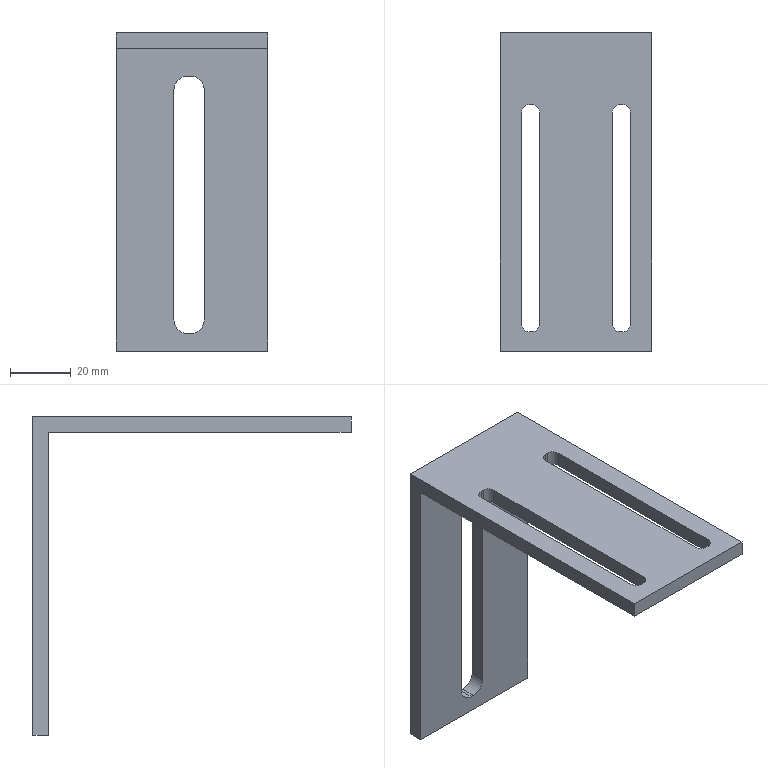Part | SolidWorks | features ICE 3, Extrusion 1 | 1 solid | 32 faces | box 50 x 105 x 105 mm | volume 42641 mm3 | plane 20 | cylinder 12 | commonest cylinder face diameters 5 x8 9 x4
STEP:
#1=CARTESIAN_POINT('',(-25.,50.,0.));
#2=VERTEX_POINT('',#1);
#3=CARTESIAN_POINT('',(-25.,-50.,0.));
#4=VERTEX_POINT('',#3);
#5=CARTESIAN_POINT('',(-25.,-50.,0.));
#6=DIRECTION('',(0.,-1.,0.));
#7=VECTOR('',#6,1000.);
#8=LINE('',#5,#7);
#9=EDGE_CURVE('',#2,#4,#8,.T.);
#10=ORIENTED_EDGE('',*,*,#9,.T.);
#11=CARTESIAN_POINT('',(-25.,-50.,5.));
#12=VERTEX_POINT('',#11);
#13=CARTESIAN_POINT('',(-25.,-50.,5.));
#14=DIRECTION('',(0.,0.,-1.));
#15=VECTOR('',#14,1000.);
#16=LINE('',#13,#15);
#17=EDGE_CURVE('',#12,#4,#16,.T.);
#18=ORIENTED_EDGE('',*,*,#17,.F.);
#19=CARTESIAN_POINT('',(-25.,55.,5.));
#20=VERTEX_POINT('',#19);
#21=CARTESIAN_POINT('',(-25.,-50.,5.));
#22=DIRECTION('',(0.,-1.,0.));
#23=VECTOR('',#22,1000.);
#24=LINE('',#21,#23);
#25=EDGE_CURVE('',#20,#12,#24,.T.);
#26=ORIENTED_EDGE('',*,*,#25,.F.);
#27=CARTESIAN_POINT('',(-25.,55.,-100.));
#28=VERTEX_POINT('',#27);
#29=CARTESIAN_POINT('',(-25.,55.,5.));
#30=DIRECTION('',(0.,0.,-1.));
#31=VECTOR('',#30,1000.);
#32=LINE('',#29,#31);
#33=EDGE_CURVE('',#20,#28,#32,.T.);
#34=ORIENTED_EDGE('',*,*,#33,.T.);
#35=CARTESIAN_POINT('',(-25.,50.,-100.));
#36=VERTEX_POINT('',#35);
#37=CARTESIAN_POINT('',(-25.,50.,-100.));
#38=DIRECTION('',(0.,1.,0.));
#39=VECTOR('',#38,1000.);
#40=LINE('',#37,#39);
#41=EDGE_CURVE('',#36,#28,#40,.T.);
#42=ORIENTED_EDGE('',*,*,#41,.F.);
#43=CARTESIAN_POINT('',(-25.,50.,5.));
#44=DIRECTION('',(0.,0.,-1.));
#45=VECTOR('',#44,1000.);
#46=LINE('',#43,#45);
#47=EDGE_CURVE('',#2,#36,#46,.T.);
#48=ORIENTED_EDGE('',*,*,#47,.F.);
#49=EDGE_LOOP('',(#10,#18,#26,#34,#42,#48));
#50=FACE_OUTER_BOUND('',#49,.T.);
#51=CARTESIAN_POINT('',(-25.,-50.,5.));
#52=DIRECTION('',(1.,0.,0.));
#53=DIRECTION('',(0.,0.,-1.));
#54=AXIS2_PLACEMENT_3D('',#51,#52,#53);
#55=PLANE('',#54);
#56=ADVANCED_FACE('',(#50),#55,.F.);
#57=CARTESIAN_POINT('',(25.,-50.,0.));
#58=VERTEX_POINT('',#57);
#59=CARTESIAN_POINT('',(25.,-50.,0.));
#60=DIRECTION('',(1.,0.,0.));
#61=VECTOR('',#60,1000.);
#62=LINE('',#59,#61);
#63=EDGE_CURVE('',#4,#58,#62,.T.);
#64=ORIENTED_EDGE('',*,*,#63,.T.);
#65=CARTESIAN_POINT('',(25.,-50.,5.));
#66=VERTEX_POINT('',#65);
#67=CARTESIAN_POINT('',(25.,-50.,5.));
#68=DIRECTION('',(0.,0.,-1.));
#69=VECTOR('',#68,1000.);
#70=LINE('',#67,#69);
#71=EDGE_CURVE('',#66,#58,#70,.T.);
#72=ORIENTED_EDGE('',*,*,#71,.F.);
#73=CARTESIAN_POINT('',(25.,-50.,5.));
#74=DIRECTION('',(1.,0.,0.));
#75=VECTOR('',#74,1000.);
#76=LINE('',#73,#75);
#77=EDGE_CURVE('',#12,#66,#76,.T.);
#78=ORIENTED_EDGE('',*,*,#77,.F.);
#79=ORIENTED_EDGE('',*,*,#17,.T.);
#80=EDGE_LOOP('',(#64,#72,#78,#79));
#81=FACE_OUTER_BOUND('',#80,.T.);
#82=CARTESIAN_POINT('',(25.,-50.,5.));
#83=DIRECTION('',(0.,1.,0.));
#84=DIRECTION('',(-1.,0.,0.));
#85=AXIS2_PLACEMENT_3D('',#82,#83,#84);
#86=PLANE('',#85);
#87=ADVANCED_FACE('',(#81),#86,.F.);
#88=CARTESIAN_POINT('',(25.,50.,0.));
#89=VERTEX_POINT('',#88);
#90=CARTESIAN_POINT('',(25.,-50.,0.));
#91=DIRECTION('',(0.,1.,0.));
#92=VECTOR('',#91,1000.);
#93=LINE('',#90,#92);
#94=EDGE_CURVE('',#58,#89,#93,.T.);
#95=ORIENTED_EDGE('',*,*,#94,.T.);
#96=CARTESIAN_POINT('',(25.,50.,-100.));
#97=VERTEX_POINT('',#96);
#98=CARTESIAN_POINT('',(25.,50.,5.));
#99=DIRECTION('',(0.,0.,-1.));
#100=VECTOR('',#99,1000.);
#101=LINE('',#98,#100);
#102=EDGE_CURVE('',#89,#97,#101,.T.);
#103=ORIENTED_EDGE('',*,*,#102,.T.);
#104=CARTESIAN_POINT('',(25.,55.,-100.));
#105=VERTEX_POINT('',#104);
#106=CARTESIAN_POINT('',(25.,50.,-100.));
#107=DIRECTION('',(0.,-1.,0.));
#108=VECTOR('',#107,1000.);
#109=LINE('',#106,#108);
#110=EDGE_CURVE('',#105,#97,#109,.T.);
#111=ORIENTED_EDGE('',*,*,#110,.F.);
#112=CARTESIAN_POINT('',(25.,55.,5.));
#113=VERTEX_POINT('',#112);
#114=CARTESIAN_POINT('',(25.,55.,5.));
#115=DIRECTION('',(0.,0.,-1.));
#116=VECTOR('',#115,1000.);
#117=LINE('',#114,#116);
#118=EDGE_CURVE('',#113,#105,#117,.T.);
#119=ORIENTED_EDGE('',*,*,#118,.F.);
#120=CARTESIAN_POINT('',(25.,-50.,5.));
#121=DIRECTION('',(0.,1.,0.));
#122=VECTOR('',#121,1000.);
#123=LINE('',#120,#122);
#124=EDGE_CURVE('',#66,#113,#123,.T.);
#125=ORIENTED_EDGE('',*,*,#124,.F.);
#126=ORIENTED_EDGE('',*,*,#71,.T.);
#127=EDGE_LOOP('',(#95,#103,#111,#119,#125,#126));
#128=FACE_OUTER_BOUND('',#127,.T.);
#129=CARTESIAN_POINT('',(25.,-50.,5.));
#130=DIRECTION('',(-1.,0.,0.));
#131=DIRECTION('',(0.,0.,1.));
#132=AXIS2_PLACEMENT_3D('',#129,#130,#131);
#133=PLANE('',#132);
#134=ADVANCED_FACE('',(#128),#133,.F.);
#135=CARTESIAN_POINT('',(-18.,-41.155,5.));
#136=VERTEX_POINT('',#135);
#137=CARTESIAN_POINT('',(-15.5,-43.655,5.));
#138=VERTEX_POINT('',#137);
#139=CARTESIAN_POINT('',(-15.5,-41.155,5.));
#140=DIRECTION('',(0.,0.,1.));
#141=DIRECTION('',(-1.,0.,0.));
#142=AXIS2_PLACEMENT_3D('',#139,#140,#141);
#143=CIRCLE('',#142,2.5);
#144=EDGE_CURVE('',#136,#138,#143,.T.);
#145=ORIENTED_EDGE('',*,*,#144,.F.);
#146=CARTESIAN_POINT('',(-18.,28.845,5.));
#147=VERTEX_POINT('',#146);
#148=CARTESIAN_POINT('',(-18.,-41.155,5.));
#149=DIRECTION('',(0.,-1.,0.));
#150=VECTOR('',#149,1000.);
#151=LINE('',#148,#150);
#152=EDGE_CURVE('',#147,#136,#151,.T.);
#153=ORIENTED_EDGE('',*,*,#152,.F.);
#154=CARTESIAN_POINT('',(-15.5,31.345,5.));
#155=VERTEX_POINT('',#154);
#156=CARTESIAN_POINT('',(-15.5,28.845,5.));
#157=DIRECTION('',(0.,0.,1.));
#158=DIRECTION('',(1.,0.,0.));
#159=AXIS2_PLACEMENT_3D('',#156,#157,#158);
#160=CIRCLE('',#159,2.5);
#161=EDGE_CURVE('',#155,#147,#160,.T.);
#162=ORIENTED_EDGE('',*,*,#161,.F.);
#163=CARTESIAN_POINT('',(-14.5,31.345,5.));
#164=VERTEX_POINT('',#163);
#165=CARTESIAN_POINT('',(-14.5,31.345,5.));
#166=DIRECTION('',(-1.,0.,0.));
#167=VECTOR('',#166,1000.);
#168=LINE('',#165,#167);
#169=EDGE_CURVE('',#164,#155,#168,.T.);
#170=ORIENTED_EDGE('',*,*,#169,.F.);
#171=CARTESIAN_POINT('',(-12.,28.845,5.));
#172=VERTEX_POINT('',#171);
#173=CARTESIAN_POINT('',(-14.5,28.845,5.));
#174=DIRECTION('',(0.,0.,1.));
#175=DIRECTION('',(1.,0.,0.));
#176=AXIS2_PLACEMENT_3D('',#173,#174,#175);
#177=CIRCLE('',#176,2.5);
#178=EDGE_CURVE('',#172,#164,#177,.T.);
#179=ORIENTED_EDGE('',*,*,#178,.F.);
#180=CARTESIAN_POINT('',(-12.,-41.155,5.));
#181=VERTEX_POINT('',#180);
#182=CARTESIAN_POINT('',(-12.,-41.155,5.));
#183=DIRECTION('',(0.,1.,0.));
#184=VECTOR('',#183,1000.);
#185=LINE('',#182,#184);
#186=EDGE_CURVE('',#181,#172,#185,.T.);
#187=ORIENTED_EDGE('',*,*,#186,.F.);
#188=CARTESIAN_POINT('',(-14.5,-43.655,5.));
#189=VERTEX_POINT('',#188);
#190=CARTESIAN_POINT('',(-14.5,-41.155,5.));
#191=DIRECTION('',(0.,0.,1.));
#192=DIRECTION('',(1.,0.,0.));
#193=AXIS2_PLACEMENT_3D('',#190,#191,#192);
#194=CIRCLE('',#193,2.5);
#195=EDGE_CURVE('',#189,#181,#194,.T.);
#196=ORIENTED_EDGE('',*,*,#195,.F.);
#197=CARTESIAN_POINT('',(-14.5,-43.655,5.));
#198=DIRECTION('',(1.,0.,0.));
#199=VECTOR('',#198,1000.);
#200=LINE('',#197,#199);
#201=EDGE_CURVE('',#138,#189,#200,.T.);
#202=ORIENTED_EDGE('',*,*,#201,.F.);
#203=EDGE_LOOP('',(#145,#153,#162,#170,#179,#187,#196,#202));
#204=FACE_BOUND('',#203,.T.);
#205=CARTESIAN_POINT('',(14.5,31.345,5.));
#206=VERTEX_POINT('',#205);
#207=CARTESIAN_POINT('',(12.,28.845,5.));
#208=VERTEX_POINT('',#207);
#209=CARTESIAN_POINT('',(14.5,28.845,5.));
#210=DIRECTION('',(0.,0.,1.));
#211=DIRECTION('',(1.,0.,0.));
#212=AXIS2_PLACEMENT_3D('',#209,#210,#211);
#213=CIRCLE('',#212,2.5);
#214=EDGE_CURVE('',#206,#208,#213,.T.);
#215=ORIENTED_EDGE('',*,*,#214,.F.);
#216=CARTESIAN_POINT('',(15.5,31.345,5.));
#217=VERTEX_POINT('',#216);
#218=CARTESIAN_POINT('',(15.5,31.345,5.));
#219=DIRECTION('',(-1.,0.,0.));
#220=VECTOR('',#219,1000.);
#221=LINE('',#218,#220);
#222=EDGE_CURVE('',#217,#206,#221,.T.);
#223=ORIENTED_EDGE('',*,*,#222,.F.);
#224=CARTESIAN_POINT('',(18.,28.845,5.));
#225=VERTEX_POINT('',#224);
#226=CARTESIAN_POINT('',(15.5,28.845,5.));
#227=DIRECTION('',(0.,0.,1.));
#228=DIRECTION('',(1.,0.,0.));
#229=AXIS2_PLACEMENT_3D('',#226,#227,#228);
#230=CIRCLE('',#229,2.5);
#231=EDGE_CURVE('',#225,#217,#230,.T.);
#232=ORIENTED_EDGE('',*,*,#231,.F.);
#233=CARTESIAN_POINT('',(18.,-41.155,5.));
#234=VERTEX_POINT('',#233);
#235=CARTESIAN_POINT('',(18.,-41.155,5.));
#236=DIRECTION('',(0.,1.,0.));
#237=VECTOR('',#236,1000.);
#238=LINE('',#235,#237);
#239=EDGE_CURVE('',#234,#225,#238,.T.);
#240=ORIENTED_EDGE('',*,*,#239,.F.);
#241=CARTESIAN_POINT('',(15.5,-43.655,5.));
#242=VERTEX_POINT('',#241);
#243=CARTESIAN_POINT('',(15.5,-41.155,5.));
#244=DIRECTION('',(0.,0.,1.));
#245=DIRECTION('',(1.,0.,0.));
#246=AXIS2_PLACEMENT_3D('',#243,#244,#245);
#247=CIRCLE('',#246,2.5);
#248=EDGE_CURVE('',#242,#234,#247,.T.);
#249=ORIENTED_EDGE('',*,*,#248,.F.);
#250=CARTESIAN_POINT('',(14.5,-43.655,5.));
#251=VERTEX_POINT('',#250);
#252=CARTESIAN_POINT('',(15.5,-43.655,5.));
#253=DIRECTION('',(1.,0.,0.));
#254=VECTOR('',#253,1000.);
#255=LINE('',#252,#254);
#256=EDGE_CURVE('',#251,#242,#255,.T.);
#257=ORIENTED_EDGE('',*,*,#256,.F.);
#258=CARTESIAN_POINT('',(12.,-41.155,5.));
#259=VERTEX_POINT('',#258);
#260=CARTESIAN_POINT('',(14.5,-41.155,5.));
#261=DIRECTION('',(0.,0.,1.));
#262=DIRECTION('',(-1.,0.,0.));
#263=AXIS2_PLACEMENT_3D('',#260,#261,#262);
#264=CIRCLE('',#263,2.5);
#265=EDGE_CURVE('',#259,#251,#264,.T.);
#266=ORIENTED_EDGE('',*,*,#265,.F.);
#267=CARTESIAN_POINT('',(12.,-41.155,5.));
#268=DIRECTION('',(0.,-1.,0.));
#269=VECTOR('',#268,1000.);
#270=LINE('',#267,#269);
#271=EDGE_CURVE('',#208,#259,#270,.T.);
#272=ORIENTED_EDGE('',*,*,#271,.F.);
#273=EDGE_LOOP('',(#215,#223,#232,#240,#249,#257,#266,#272));
#274=FACE_BOUND('',#273,.T.);
#275=ORIENTED_EDGE('',*,*,#25,.T.);
#276=ORIENTED_EDGE('',*,*,#77,.T.);
#277=ORIENTED_EDGE('',*,*,#124,.T.);
#278=CARTESIAN_POINT('',(-25.,55.,5.));
#279=DIRECTION('',(1.,0.,0.));
#280=VECTOR('',#279,1000.);
#281=LINE('',#278,#280);
#282=EDGE_CURVE('',#20,#113,#281,.T.);
#283=ORIENTED_EDGE('',*,*,#282,.F.);
#284=EDGE_LOOP('',(#275,#276,#277,#283));
#285=FACE_OUTER_BOUND('',#284,.T.);
#286=CARTESIAN_POINT('',(-25.,50.,5.));
#287=DIRECTION('',(0.,0.,1.));
#288=DIRECTION('',(1.,0.,0.));
#289=AXIS2_PLACEMENT_3D('',#286,#287,#288);
#290=PLANE('',#289);
#291=ADVANCED_FACE('',(#204,#274,#285),#290,.T.);
#292=CARTESIAN_POINT('',(-18.,28.845,0.));
#293=VERTEX_POINT('',#292);
#294=CARTESIAN_POINT('',(-18.,-41.155,0.));
#295=VERTEX_POINT('',#294);
#296=CARTESIAN_POINT('',(-18.,50.,0.));
#297=DIRECTION('',(0.,-1.,0.));
#298=VECTOR('',#297,1000.);
#299=LINE('',#296,#298);
#300=EDGE_CURVE('',#293,#295,#299,.T.);
#301=ORIENTED_EDGE('',*,*,#300,.T.);
#302=CARTESIAN_POINT('',(-15.5,-43.655,0.));
#303=VERTEX_POINT('',#302);
#304=CARTESIAN_POINT('',(-15.5,-41.155,0.));
#305=DIRECTION('',(0.,0.,1.));
#306=DIRECTION('',(1.,0.,0.));
#307=AXIS2_PLACEMENT_3D('',#304,#305,#306);
#308=CIRCLE('',#307,2.5);
#309=EDGE_CURVE('',#295,#303,#308,.T.);
#310=ORIENTED_EDGE('',*,*,#309,.T.);
#311=CARTESIAN_POINT('',(-14.5,-43.655,0.));
#312=VERTEX_POINT('',#311);
#313=CARTESIAN_POINT('',(-25.,-43.655,0.));
#314=DIRECTION('',(1.,0.,0.));
#315=VECTOR('',#314,1000.);
#316=LINE('',#313,#315);
#317=EDGE_CURVE('',#303,#312,#316,.T.);
#318=ORIENTED_EDGE('',*,*,#317,.T.);
#319=CARTESIAN_POINT('',(-12.,-41.155,0.));
#320=VERTEX_POINT('',#319);
#321=CARTESIAN_POINT('',(-14.5,-41.155,0.));
#322=DIRECTION('',(0.,0.,1.));
#323=DIRECTION('',(1.,0.,0.));
#324=AXIS2_PLACEMENT_3D('',#321,#322,#323);
#325=CIRCLE('',#324,2.5);
#326=EDGE_CURVE('',#312,#320,#325,.T.);
#327=ORIENTED_EDGE('',*,*,#326,.T.);
#328=CARTESIAN_POINT('',(-12.,28.845,0.));
#329=VERTEX_POINT('',#328);
#330=CARTESIAN_POINT('',(-12.,50.,0.));
#331=DIRECTION('',(0.,1.,0.));
#332=VECTOR('',#331,1000.);
#333=LINE('',#330,#332);
#334=EDGE_CURVE('',#320,#329,#333,.T.);
#335=ORIENTED_EDGE('',*,*,#334,.T.);
#336=CARTESIAN_POINT('',(-14.5,31.345,0.));
#337=VERTEX_POINT('',#336);
#338=CARTESIAN_POINT('',(-14.5,28.845,0.));
#339=DIRECTION('',(0.,0.,1.));
#340=DIRECTION('',(1.,0.,0.));
#341=AXIS2_PLACEMENT_3D('',#338,#339,#340);
#342=CIRCLE('',#341,2.5);
#343=EDGE_CURVE('',#329,#337,#342,.T.);
#344=ORIENTED_EDGE('',*,*,#343,.T.);
#345=CARTESIAN_POINT('',(-15.5,31.345,0.));
#346=VERTEX_POINT('',#345);
#347=CARTESIAN_POINT('',(-25.,31.345,0.));
#348=DIRECTION('',(-1.,0.,0.));
#349=VECTOR('',#348,1000.);
#350=LINE('',#347,#349);
#351=EDGE_CURVE('',#337,#346,#350,.T.);
#352=ORIENTED_EDGE('',*,*,#351,.T.);
#353=CARTESIAN_POINT('',(-15.5,28.845,0.));
#354=DIRECTION('',(0.,0.,1.));
#355=DIRECTION('',(1.,0.,0.));
#356=AXIS2_PLACEMENT_3D('',#353,#354,#355);
#357=CIRCLE('',#356,2.5);
#358=EDGE_CURVE('',#346,#293,#357,.T.);
#359=ORIENTED_EDGE('',*,*,#358,.T.);
#360=EDGE_LOOP('',(#301,#310,#318,#327,#335,#344,#352,#359));
#361=FACE_BOUND('',#360,.T.);
#362=CARTESIAN_POINT('',(15.5,31.345,0.));
#363=VERTEX_POINT('',#362);
#364=CARTESIAN_POINT('',(14.5,31.345,0.));
#365=VERTEX_POINT('',#364);
#366=CARTESIAN_POINT('',(-25.,31.345,0.));
#367=DIRECTION('',(-1.,0.,0.));
#368=VECTOR('',#367,1000.);
#369=LINE('',#366,#368);
#370=EDGE_CURVE('',#363,#365,#369,.T.);
#371=ORIENTED_EDGE('',*,*,#370,.T.);
#372=CARTESIAN_POINT('',(12.,28.845,0.));
#373=VERTEX_POINT('',#372);
#374=CARTESIAN_POINT('',(14.5,28.845,0.));
#375=DIRECTION('',(0.,0.,1.));
#376=DIRECTION('',(1.,0.,0.));
#377=AXIS2_PLACEMENT_3D('',#374,#375,#376);
#378=CIRCLE('',#377,2.5);
#379=EDGE_CURVE('',#365,#373,#378,.T.);
#380=ORIENTED_EDGE('',*,*,#379,.T.);
#381=CARTESIAN_POINT('',(12.,-41.155,0.));
#382=VERTEX_POINT('',#381);
#383=CARTESIAN_POINT('',(12.,50.,0.));
#384=DIRECTION('',(0.,-1.,0.));
#385=VECTOR('',#384,1000.);
#386=LINE('',#383,#385);
#387=EDGE_CURVE('',#373,#382,#386,.T.);
#388=ORIENTED_EDGE('',*,*,#387,.T.);
#389=CARTESIAN_POINT('',(14.5,-43.655,0.));
#390=VERTEX_POINT('',#389);
#391=CARTESIAN_POINT('',(14.5,-41.155,0.));
#392=DIRECTION('',(0.,0.,1.));
#393=DIRECTION('',(1.,0.,0.));
#394=AXIS2_PLACEMENT_3D('',#391,#392,#393);
#395=CIRCLE('',#394,2.5);
#396=EDGE_CURVE('',#382,#390,#395,.T.);
#397=ORIENTED_EDGE('',*,*,#396,.T.);
#398=CARTESIAN_POINT('',(15.5,-43.655,0.));
#399=VERTEX_POINT('',#398);
#400=CARTESIAN_POINT('',(-25.,-43.655,0.));
#401=DIRECTION('',(1.,0.,0.));
#402=VECTOR('',#401,1000.);
#403=LINE('',#400,#402);
#404=EDGE_CURVE('',#390,#399,#403,.T.);
#405=ORIENTED_EDGE('',*,*,#404,.T.);
#406=CARTESIAN_POINT('',(18.,-41.155,0.));
#407=VERTEX_POINT('',#406);
#408=CARTESIAN_POINT('',(15.5,-41.155,0.));
#409=DIRECTION('',(0.,0.,1.));
#410=DIRECTION('',(1.,0.,0.));
#411=AXIS2_PLACEMENT_3D('',#408,#409,#410);
#412=CIRCLE('',#411,2.5);
#413=EDGE_CURVE('',#399,#407,#412,.T.);
#414=ORIENTED_EDGE('',*,*,#413,.T.);
#415=CARTESIAN_POINT('',(18.,28.845,0.));
#416=VERTEX_POINT('',#415);
#417=CARTESIAN_POINT('',(18.,50.,0.));
#418=DIRECTION('',(0.,1.,0.));
#419=VECTOR('',#418,1000.);
#420=LINE('',#417,#419);
#421=EDGE_CURVE('',#407,#416,#420,.T.);
#422=ORIENTED_EDGE('',*,*,#421,.T.);
#423=CARTESIAN_POINT('',(15.5,28.845,0.));
#424=DIRECTION('',(0.,0.,1.));
#425=DIRECTION('',(1.,0.,0.));
#426=AXIS2_PLACEMENT_3D('',#423,#424,#425);
#427=CIRCLE('',#426,2.5);
#428=EDGE_CURVE('',#416,#363,#427,.T.);
#429=ORIENTED_EDGE('',*,*,#428,.T.);
#430=EDGE_LOOP('',(#371,#380,#388,#397,#405,#414,#422,#429));
#431=FACE_BOUND('',#430,.T.);
#432=ORIENTED_EDGE('',*,*,#9,.F.);
#433=CARTESIAN_POINT('',(25.,50.,0.));
#434=DIRECTION('',(-1.,0.,0.));
#435=VECTOR('',#434,1000.);
#436=LINE('',#433,#435);
#437=EDGE_CURVE('',#89,#2,#436,.T.);
#438=ORIENTED_EDGE('',*,*,#437,.F.);
#439=ORIENTED_EDGE('',*,*,#94,.F.);
#440=ORIENTED_EDGE('',*,*,#63,.F.);
#441=EDGE_LOOP('',(#432,#438,#439,#440));
#442=FACE_OUTER_BOUND('',#441,.T.);
#443=CARTESIAN_POINT('',(-25.,50.,0.));
#444=DIRECTION('',(0.,0.,1.));
#445=DIRECTION('',(1.,0.,0.));
#446=AXIS2_PLACEMENT_3D('',#443,#444,#445);
#447=PLANE('',#446);
#448=ADVANCED_FACE('',(#361,#431,#442),#447,.F.);
#449=CARTESIAN_POINT('',(14.5,31.345,-5.));
#450=DIRECTION('',(0.,0.,1.));
#451=VECTOR('',#450,1000.);
#452=LINE('',#449,#451);
#453=EDGE_CURVE('',#365,#206,#452,.T.);
#454=ORIENTED_EDGE('',*,*,#453,.T.);
#455=ORIENTED_EDGE('',*,*,#214,.T.);
#456=CARTESIAN_POINT('',(12.,28.845,-5.));
#457=DIRECTION('',(0.,0.,1.));
#458=VECTOR('',#457,1000.);
#459=LINE('',#456,#458);
#460=EDGE_CURVE('',#373,#208,#459,.T.);
#461=ORIENTED_EDGE('',*,*,#460,.F.);
#462=ORIENTED_EDGE('',*,*,#379,.F.);
#463=EDGE_LOOP('',(#454,#455,#461,#462));
#464=FACE_OUTER_BOUND('',#463,.T.);
#465=CARTESIAN_POINT('',(14.5,28.845,-5.));
#466=DIRECTION('',(0.,0.,1.));
#467=DIRECTION('',(1.,0.,0.));
#468=AXIS2_PLACEMENT_3D('',#465,#466,#467);
#469=CYLINDRICAL_SURFACE('',#468,2.5);
#470=ADVANCED_FACE('',(#464),#469,.F.);
#471=CARTESIAN_POINT('',(15.5,31.345,-5.));
#472=DIRECTION('',(0.,0.,1.));
#473=VECTOR('',#472,1000.);
#474=LINE('',#471,#473);
#475=EDGE_CURVE('',#363,#217,#474,.T.);
#476=ORIENTED_EDGE('',*,*,#475,.T.);
#477=ORIENTED_EDGE('',*,*,#222,.T.);
#478=ORIENTED_EDGE('',*,*,#453,.F.);
#479=ORIENTED_EDGE('',*,*,#370,.F.);
#480=EDGE_LOOP('',(#476,#477,#478,#479));
#481=FACE_OUTER_BOUND('',#480,.T.);
#482=CARTESIAN_POINT('',(15.5,31.345,-5.));
#483=DIRECTION('',(0.,1.,0.));
#484=DIRECTION('',(0.,0.,1.));
#485=AXIS2_PLACEMENT_3D('',#482,#483,#484);
#486=PLANE('',#485);
#487=ADVANCED_FACE('',(#481),#486,.F.);
#488=CARTESIAN_POINT('',(18.,28.845,-5.));
#489=DIRECTION('',(0.,0.,1.));
#490=VECTOR('',#489,1000.);
#491=LINE('',#488,#490);
#492=EDGE_CURVE('',#416,#225,#491,.T.);
#493=ORIENTED_EDGE('',*,*,#492,.T.);
#494=ORIENTED_EDGE('',*,*,#231,.T.);
#495=ORIENTED_EDGE('',*,*,#475,.F.);
#496=ORIENTED_EDGE('',*,*,#428,.F.);
#497=EDGE_LOOP('',(#493,#494,#495,#496));
#498=FACE_OUTER_BOUND('',#497,.T.);
#499=CARTESIAN_POINT('',(15.5,28.845,-5.));
#500=DIRECTION('',(0.,0.,1.));
#501=DIRECTION('',(1.,0.,0.));
#502=AXIS2_PLACEMENT_3D('',#499,#500,#501);
#503=CYLINDRICAL_SURFACE('',#502,2.5);
#504=ADVANCED_FACE('',(#498),#503,.F.);
#505=CARTESIAN_POINT('',(18.,-41.155,-5.));
#506=DIRECTION('',(0.,0.,1.));
#507=VECTOR('',#506,1000.);
#508=LINE('',#505,#507);
#509=EDGE_CURVE('',#407,#234,#508,.T.);
#510=ORIENTED_EDGE('',*,*,#509,.T.);
#511=ORIENTED_EDGE('',*,*,#239,.T.);
#512=ORIENTED_EDGE('',*,*,#492,.F.);
#513=ORIENTED_EDGE('',*,*,#421,.F.);
#514=EDGE_LOOP('',(#510,#511,#512,#513));
#515=FACE_OUTER_BOUND('',#514,.T.);
#516=CARTESIAN_POINT('',(18.,-41.155,-5.));
#517=DIRECTION('',(1.,0.,0.));
#518=DIRECTION('',(0.,0.,-1.));
#519=AXIS2_PLACEMENT_3D('',#516,#517,#518);
#520=PLANE('',#519);
#521=ADVANCED_FACE('',(#515),#520,.F.);
#522=CARTESIAN_POINT('',(15.5,-43.655,-5.));
#523=DIRECTION('',(0.,0.,1.));
#524=VECTOR('',#523,1000.);
#525=LINE('',#522,#524);
#526=EDGE_CURVE('',#399,#242,#525,.T.);
#527=ORIENTED_EDGE('',*,*,#526,.T.);
#528=ORIENTED_EDGE('',*,*,#248,.T.);
#529=ORIENTED_EDGE('',*,*,#509,.F.);
#530=ORIENTED_EDGE('',*,*,#413,.F.);
#531=EDGE_LOOP('',(#527,#528,#529,#530));
#532=FACE_OUTER_BOUND('',#531,.T.);
#533=CARTESIAN_POINT('',(15.5,-41.155,-5.));
#534=DIRECTION('',(0.,0.,1.));
#535=DIRECTION('',(1.,0.,0.));
#536=AXIS2_PLACEMENT_3D('',#533,#534,#535);
#537=CYLINDRICAL_SURFACE('',#536,2.5);
#538=ADVANCED_FACE('',(#532),#537,.F.);
#539=CARTESIAN_POINT('',(14.5,-43.655,-5.));
#540=DIRECTION('',(0.,0.,1.));
#541=VECTOR('',#540,1000.);
#542=LINE('',#539,#541);
#543=EDGE_CURVE('',#390,#251,#542,.T.);
#544=ORIENTED_EDGE('',*,*,#543,.T.);
#545=ORIENTED_EDGE('',*,*,#256,.T.);
#546=ORIENTED_EDGE('',*,*,#526,.F.);
#547=ORIENTED_EDGE('',*,*,#404,.F.);
#548=EDGE_LOOP('',(#544,#545,#546,#547));
#549=FACE_OUTER_BOUND('',#548,.T.);
#550=CARTESIAN_POINT('',(15.5,-43.655,-5.));
#551=DIRECTION('',(0.,-1.,0.));
#552=DIRECTION('',(0.,0.,-1.));
#553=AXIS2_PLACEMENT_3D('',#550,#551,#552);
#554=PLANE('',#553);
#555=ADVANCED_FACE('',(#549),#554,.F.);
#556=CARTESIAN_POINT('',(12.,-41.155,-5.));
#557=DIRECTION('',(0.,0.,1.));
#558=VECTOR('',#557,1000.);
#559=LINE('',#556,#558);
#560=EDGE_CURVE('',#382,#259,#559,.T.);
#561=ORIENTED_EDGE('',*,*,#560,.T.);
#562=ORIENTED_EDGE('',*,*,#265,.T.);
#563=ORIENTED_EDGE('',*,*,#543,.F.);
#564=ORIENTED_EDGE('',*,*,#396,.F.);
#565=EDGE_LOOP('',(#561,#562,#563,#564));
#566=FACE_OUTER_BOUND('',#565,.T.);
#567=CARTESIAN_POINT('',(14.5,-41.155,-5.));
#568=DIRECTION('',(0.,0.,1.));
#569=DIRECTION('',(1.,0.,0.));
#570=AXIS2_PLACEMENT_3D('',#567,#568,#569);
#571=CYLINDRICAL_SURFACE('',#570,2.5);
#572=ADVANCED_FACE('',(#566),#571,.F.);
#573=ORIENTED_EDGE('',*,*,#460,.T.);
#574=ORIENTED_EDGE('',*,*,#271,.T.);
#575=ORIENTED_EDGE('',*,*,#560,.F.);
#576=ORIENTED_EDGE('',*,*,#387,.F.);
#577=EDGE_LOOP('',(#573,#574,#575,#576));
#578=FACE_OUTER_BOUND('',#577,.T.);
#579=CARTESIAN_POINT('',(12.,-41.155,-5.));
#580=DIRECTION('',(-1.,0.,0.));
#581=DIRECTION('',(0.,0.,1.));
#582=AXIS2_PLACEMENT_3D('',#579,#580,#581);
#583=PLANE('',#582);
#584=ADVANCED_FACE('',(#578),#583,.F.);
#585=CARTESIAN_POINT('',(-18.,-41.155,-5.));
#586=DIRECTION('',(0.,0.,1.));
#587=VECTOR('',#586,1000.);
#588=LINE('',#585,#587);
#589=EDGE_CURVE('',#295,#136,#588,.T.);
#590=ORIENTED_EDGE('',*,*,#589,.T.);
#591=ORIENTED_EDGE('',*,*,#144,.T.);
#592=CARTESIAN_POINT('',(-15.5,-43.655,-5.));
#593=DIRECTION('',(0.,0.,1.));
#594=VECTOR('',#593,1000.);
#595=LINE('',#592,#594);
#596=EDGE_CURVE('',#303,#138,#595,.T.);
#597=ORIENTED_EDGE('',*,*,#596,.F.);
#598=ORIENTED_EDGE('',*,*,#309,.F.);
#599=EDGE_LOOP('',(#590,#591,#597,#598));
#600=FACE_OUTER_BOUND('',#599,.T.);
#601=CARTESIAN_POINT('',(-15.5,-41.155,-5.));
#602=DIRECTION('',(0.,0.,1.));
#603=DIRECTION('',(1.,0.,0.));
#604=AXIS2_PLACEMENT_3D('',#601,#602,#603);
#605=CYLINDRICAL_SURFACE('',#604,2.5);
#606=ADVANCED_FACE('',(#600),#605,.F.);
#607=CARTESIAN_POINT('',(-18.,28.845,-5.));
#608=DIRECTION('',(0.,0.,1.));
#609=VECTOR('',#608,1000.);
#610=LINE('',#607,#609);
#611=EDGE_CURVE('',#293,#147,#610,.T.);
#612=ORIENTED_EDGE('',*,*,#611,.T.);
#613=ORIENTED_EDGE('',*,*,#152,.T.);
#614=ORIENTED_EDGE('',*,*,#589,.F.);
#615=ORIENTED_EDGE('',*,*,#300,.F.);
#616=EDGE_LOOP('',(#612,#613,#614,#615));
#617=FACE_OUTER_BOUND('',#616,.T.);
#618=CARTESIAN_POINT('',(-18.,-41.155,-5.));
#619=DIRECTION('',(-1.,0.,0.));
#620=DIRECTION('',(0.,0.,1.));
#621=AXIS2_PLACEMENT_3D('',#618,#619,#620);
#622=PLANE('',#621);
#623=ADVANCED_FACE('',(#617),#622,.F.);
#624=CARTESIAN_POINT('',(-15.5,31.345,-5.));
#625=DIRECTION('',(0.,0.,1.));
#626=VECTOR('',#625,1000.);
#627=LINE('',#624,#626);
#628=EDGE_CURVE('',#346,#155,#627,.T.);
#629=ORIENTED_EDGE('',*,*,#628,.T.);
#630=ORIENTED_EDGE('',*,*,#161,.T.);
#631=ORIENTED_EDGE('',*,*,#611,.F.);
#632=ORIENTED_EDGE('',*,*,#358,.F.);
#633=EDGE_LOOP('',(#629,#630,#631,#632));
#634=FACE_OUTER_BOUND('',#633,.T.);
#635=CARTESIAN_POINT('',(-15.5,28.845,-5.));
#636=DIRECTION('',(0.,0.,1.));
#637=DIRECTION('',(1.,0.,0.));
#638=AXIS2_PLACEMENT_3D('',#635,#636,#637);
#639=CYLINDRICAL_SURFACE('',#638,2.5);
#640=ADVANCED_FACE('',(#634),#639,.F.);
#641=CARTESIAN_POINT('',(-14.5,31.345,-5.));
#642=DIRECTION('',(0.,0.,1.));
#643=VECTOR('',#642,1000.);
#644=LINE('',#641,#643);
#645=EDGE_CURVE('',#337,#164,#644,.T.);
#646=ORIENTED_EDGE('',*,*,#645,.T.);
#647=ORIENTED_EDGE('',*,*,#169,.T.);
#648=ORIENTED_EDGE('',*,*,#628,.F.);
#649=ORIENTED_EDGE('',*,*,#351,.F.);
#650=EDGE_LOOP('',(#646,#647,#648,#649));
#651=FACE_OUTER_BOUND('',#650,.T.);
#652=CARTESIAN_POINT('',(-14.5,31.345,-5.));
#653=DIRECTION('',(0.,1.,0.));
#654=DIRECTION('',(0.,0.,1.));
#655=AXIS2_PLACEMENT_3D('',#652,#653,#654);
#656=PLANE('',#655);
#657=ADVANCED_FACE('',(#651),#656,.F.);
#658=CARTESIAN_POINT('',(-12.,28.845,-5.));
#659=DIRECTION('',(0.,0.,1.));
#660=VECTOR('',#659,1000.);
#661=LINE('',#658,#660);
#662=EDGE_CURVE('',#329,#172,#661,.T.);
#663=ORIENTED_EDGE('',*,*,#662,.T.);
#664=ORIENTED_EDGE('',*,*,#178,.T.);
#665=ORIENTED_EDGE('',*,*,#645,.F.);
#666=ORIENTED_EDGE('',*,*,#343,.F.);
#667=EDGE_LOOP('',(#663,#664,#665,#666));
#668=FACE_OUTER_BOUND('',#667,.T.);
#669=CARTESIAN_POINT('',(-14.5,28.845,-5.));
#670=DIRECTION('',(0.,0.,1.));
#671=DIRECTION('',(1.,0.,0.));
#672=AXIS2_PLACEMENT_3D('',#669,#670,#671);
#673=CYLINDRICAL_SURFACE('',#672,2.5);
#674=ADVANCED_FACE('',(#668),#673,.F.);
#675=CARTESIAN_POINT('',(-12.,-41.155,-5.));
#676=DIRECTION('',(0.,0.,1.));
#677=VECTOR('',#676,1000.);
#678=LINE('',#675,#677);
#679=EDGE_CURVE('',#320,#181,#678,.T.);
#680=ORIENTED_EDGE('',*,*,#679,.T.);
#681=ORIENTED_EDGE('',*,*,#186,.T.);
#682=ORIENTED_EDGE('',*,*,#662,.F.);
#683=ORIENTED_EDGE('',*,*,#334,.F.);
#684=EDGE_LOOP('',(#680,#681,#682,#683));
#685=FACE_OUTER_BOUND('',#684,.T.);
#686=CARTESIAN_POINT('',(-12.,-41.155,-5.));
#687=DIRECTION('',(1.,0.,0.));
#688=DIRECTION('',(0.,0.,-1.));
#689=AXIS2_PLACEMENT_3D('',#686,#687,#688);
#690=PLANE('',#689);
#691=ADVANCED_FACE('',(#685),#690,.F.);
#692=CARTESIAN_POINT('',(-14.5,-43.655,-5.));
#693=DIRECTION('',(0.,0.,1.));
#694=VECTOR('',#693,1000.);
#695=LINE('',#692,#694);
#696=EDGE_CURVE('',#312,#189,#695,.T.);
#697=ORIENTED_EDGE('',*,*,#696,.T.);
#698=ORIENTED_EDGE('',*,*,#195,.T.);
#699=ORIENTED_EDGE('',*,*,#679,.F.);
#700=ORIENTED_EDGE('',*,*,#326,.F.);
#701=EDGE_LOOP('',(#697,#698,#699,#700));
#702=FACE_OUTER_BOUND('',#701,.T.);
#703=CARTESIAN_POINT('',(-14.5,-41.155,-5.));
#704=DIRECTION('',(0.,0.,1.));
#705=DIRECTION('',(1.,0.,0.));
#706=AXIS2_PLACEMENT_3D('',#703,#704,#705);
#707=CYLINDRICAL_SURFACE('',#706,2.5);
#708=ADVANCED_FACE('',(#702),#707,.F.);
#709=ORIENTED_EDGE('',*,*,#596,.T.);
#710=ORIENTED_EDGE('',*,*,#201,.T.);
#711=ORIENTED_EDGE('',*,*,#696,.F.);
#712=ORIENTED_EDGE('',*,*,#317,.F.);
#713=EDGE_LOOP('',(#709,#710,#711,#712));
#714=FACE_OUTER_BOUND('',#713,.T.);
#715=CARTESIAN_POINT('',(-14.5,-43.655,-5.));
#716=DIRECTION('',(0.,-1.,0.));
#717=DIRECTION('',(0.,0.,-1.));
#718=AXIS2_PLACEMENT_3D('',#715,#716,#717);
#719=PLANE('',#718);
#720=ADVANCED_FACE('',(#714),#719,.F.);
#721=CARTESIAN_POINT('',(-5.974,50.,-89.753));
#722=VERTEX_POINT('',#721);
#723=CARTESIAN_POINT('',(-1.474,50.,-94.253));
#724=VERTEX_POINT('',#723);
#725=CARTESIAN_POINT('',(-1.474,50.,-89.753));
#726=DIRECTION('',(0.,-1.,0.));
#727=DIRECTION('',(-1.,0.,0.));
#728=AXIS2_PLACEMENT_3D('',#725,#726,#727);
#729=CIRCLE('',#728,4.5);
#730=EDGE_CURVE('',#722,#724,#729,.T.);
#731=ORIENTED_EDGE('',*,*,#730,.F.);
#732=CARTESIAN_POINT('',(-5.974,50.,-13.753));
#733=VERTEX_POINT('',#732);
#734=CARTESIAN_POINT('',(-5.974,50.,-89.753));
#735=DIRECTION('',(0.,0.,-1.));
#736=VECTOR('',#735,1000.);
#737=LINE('',#734,#736);
#738=EDGE_CURVE('',#733,#722,#737,.T.);
#739=ORIENTED_EDGE('',*,*,#738,.F.);
#740=CARTESIAN_POINT('',(-1.474,50.,-9.253));
#741=VERTEX_POINT('',#740);
#742=CARTESIAN_POINT('',(-1.474,50.,-13.753));
#743=DIRECTION('',(0.,-1.,0.));
#744=DIRECTION('',(1.,0.,0.));
#745=AXIS2_PLACEMENT_3D('',#742,#743,#744);
#746=CIRCLE('',#745,4.5);
#747=EDGE_CURVE('',#741,#733,#746,.T.);
#748=ORIENTED_EDGE('',*,*,#747,.F.);
#749=CARTESIAN_POINT('',(-0.474,50.,-9.253));
#750=VERTEX_POINT('',#749);
#751=CARTESIAN_POINT('',(-0.474,50.,-9.253));
#752=DIRECTION('',(-1.,0.,0.));
#753=VECTOR('',#752,1000.);
#754=LINE('',#751,#753);
#755=EDGE_CURVE('',#750,#741,#754,.T.);
#756=ORIENTED_EDGE('',*,*,#755,.F.);
#757=CARTESIAN_POINT('',(4.026,50.,-13.753));
#758=VERTEX_POINT('',#757);
#759=CARTESIAN_POINT('',(-0.474,50.,-13.753));
#760=DIRECTION('',(0.,-1.,0.));
#761=DIRECTION('',(1.,0.,0.));
#762=AXIS2_PLACEMENT_3D('',#759,#760,#761);
#763=CIRCLE('',#762,4.5);
#764=EDGE_CURVE('',#758,#750,#763,.T.);
#765=ORIENTED_EDGE('',*,*,#764,.F.);
#766=CARTESIAN_POINT('',(4.026,50.,-89.753));
#767=VERTEX_POINT('',#766);
#768=CARTESIAN_POINT('',(4.026,50.,-89.753));
#769=DIRECTION('',(0.,0.,1.));
#770=VECTOR('',#769,1000.);
#771=LINE('',#768,#770);
#772=EDGE_CURVE('',#767,#758,#771,.T.);
#773=ORIENTED_EDGE('',*,*,#772,.F.);
#774=CARTESIAN_POINT('',(-0.474,50.,-94.253));
#775=VERTEX_POINT('',#774);
#776=CARTESIAN_POINT('',(-0.474,50.,-89.753));
#777=DIRECTION('',(0.,-1.,0.));
#778=DIRECTION('',(1.,0.,0.));
#779=AXIS2_PLACEMENT_3D('',#776,#777,#778);
#780=CIRCLE('',#779,4.5);
#781=EDGE_CURVE('',#775,#767,#780,.T.);
#782=ORIENTED_EDGE('',*,*,#781,.F.);
#783=CARTESIAN_POINT('',(-0.474,50.,-94.253));
#784=DIRECTION('',(1.,0.,0.));
#785=VECTOR('',#784,1000.);
#786=LINE('',#783,#785);
#787=EDGE_CURVE('',#724,#775,#786,.T.);
#788=ORIENTED_EDGE('',*,*,#787,.F.);
#789=EDGE_LOOP('',(#731,#739,#748,#756,#765,#773,#782,#788));
#790=FACE_BOUND('',#789,.T.);
#791=ORIENTED_EDGE('',*,*,#102,.F.);
#792=ORIENTED_EDGE('',*,*,#437,.T.);
#793=ORIENTED_EDGE('',*,*,#47,.T.);
#794=CARTESIAN_POINT('',(-25.,50.,-100.));
#795=DIRECTION('',(-1.,0.,0.));
#796=VECTOR('',#795,1000.);
#797=LINE('',#794,#796);
#798=EDGE_CURVE('',#97,#36,#797,.T.);
#799=ORIENTED_EDGE('',*,*,#798,.F.);
#800=EDGE_LOOP('',(#791,#792,#793,#799));
#801=FACE_OUTER_BOUND('',#800,.T.);
#802=CARTESIAN_POINT('',(-25.,50.,5.));
#803=DIRECTION('',(0.,-1.,0.));
#804=DIRECTION('',(1.,0.,0.));
#805=AXIS2_PLACEMENT_3D('',#802,#803,#804);
#806=PLANE('',#805);
#807=ADVANCED_FACE('',(#790,#801),#806,.T.);
#808=CARTESIAN_POINT('',(-1.474,55.,-94.253));
#809=VERTEX_POINT('',#808);
#810=CARTESIAN_POINT('',(-5.974,55.,-89.753));
#811=VERTEX_POINT('',#810);
#812=CARTESIAN_POINT('',(-1.474,55.,-89.753));
#813=DIRECTION('',(0.,1.,0.));
#814=DIRECTION('',(-1.,0.,0.));
#815=AXIS2_PLACEMENT_3D('',#812,#813,#814);
#816=CIRCLE('',#815,4.5);
#817=EDGE_CURVE('',#809,#811,#816,.T.);
#818=ORIENTED_EDGE('',*,*,#817,.F.);
#819=CARTESIAN_POINT('',(-0.474,55.,-94.253));
#820=VERTEX_POINT('',#819);
#821=CARTESIAN_POINT('',(-25.,55.,-94.253));
#822=DIRECTION('',(-1.,0.,0.));
#823=VECTOR('',#822,1000.);
#824=LINE('',#821,#823);
#825=EDGE_CURVE('',#820,#809,#824,.T.);
#826=ORIENTED_EDGE('',*,*,#825,.F.);
#827=CARTESIAN_POINT('',(4.026,55.,-89.753));
#828=VERTEX_POINT('',#827);
#829=CARTESIAN_POINT('',(-0.474,55.,-89.753));
#830=DIRECTION('',(0.,1.,0.));
#831=DIRECTION('',(-1.,0.,0.));
#832=AXIS2_PLACEMENT_3D('',#829,#830,#831);
#833=CIRCLE('',#832,4.5);
#834=EDGE_CURVE('',#828,#820,#833,.T.);
#835=ORIENTED_EDGE('',*,*,#834,.F.);
#836=CARTESIAN_POINT('',(4.026,55.,-13.753));
#837=VERTEX_POINT('',#836);
#838=CARTESIAN_POINT('',(4.026,55.,5.));
#839=DIRECTION('',(0.,0.,-1.));
#840=VECTOR('',#839,1000.);
#841=LINE('',#838,#840);
#842=EDGE_CURVE('',#837,#828,#841,.T.);
#843=ORIENTED_EDGE('',*,*,#842,.F.);
#844=CARTESIAN_POINT('',(-0.474,55.,-9.253));
#845=VERTEX_POINT('',#844);
#846=CARTESIAN_POINT('',(-0.474,55.,-13.753));
#847=DIRECTION('',(0.,1.,0.));
#848=DIRECTION('',(-1.,0.,0.));
#849=AXIS2_PLACEMENT_3D('',#846,#847,#848);
#850=CIRCLE('',#849,4.5);
#851=EDGE_CURVE('',#845,#837,#850,.T.);
#852=ORIENTED_EDGE('',*,*,#851,.F.);
#853=CARTESIAN_POINT('',(-1.474,55.,-9.253));
#854=VERTEX_POINT('',#853);
#855=CARTESIAN_POINT('',(-25.,55.,-9.253));
#856=DIRECTION('',(1.,0.,0.));
#857=VECTOR('',#856,1000.);
#858=LINE('',#855,#857);
#859=EDGE_CURVE('',#854,#845,#858,.T.);
#860=ORIENTED_EDGE('',*,*,#859,.F.);
#861=CARTESIAN_POINT('',(-5.974,55.,-13.753));
#862=VERTEX_POINT('',#861);
#863=CARTESIAN_POINT('',(-1.474,55.,-13.753));
#864=DIRECTION('',(0.,1.,0.));
#865=DIRECTION('',(-1.,0.,0.));
#866=AXIS2_PLACEMENT_3D('',#863,#864,#865);
#867=CIRCLE('',#866,4.5);
#868=EDGE_CURVE('',#862,#854,#867,.T.);
#869=ORIENTED_EDGE('',*,*,#868,.F.);
#870=CARTESIAN_POINT('',(-5.974,55.,5.));
#871=DIRECTION('',(0.,0.,1.));
#872=VECTOR('',#871,1000.);
#873=LINE('',#870,#872);
#874=EDGE_CURVE('',#811,#862,#873,.T.);
#875=ORIENTED_EDGE('',*,*,#874,.F.);
#876=EDGE_LOOP('',(#818,#826,#835,#843,#852,#860,#869,#875));
#877=FACE_BOUND('',#876,.T.);
#878=ORIENTED_EDGE('',*,*,#118,.T.);
#879=CARTESIAN_POINT('',(-25.,55.,-100.));
#880=DIRECTION('',(1.,0.,0.));
#881=VECTOR('',#880,1000.);
#882=LINE('',#879,#881);
#883=EDGE_CURVE('',#28,#105,#882,.T.);
#884=ORIENTED_EDGE('',*,*,#883,.F.);
#885=ORIENTED_EDGE('',*,*,#33,.F.);
#886=ORIENTED_EDGE('',*,*,#282,.T.);
#887=EDGE_LOOP('',(#878,#884,#885,#886));
#888=FACE_OUTER_BOUND('',#887,.T.);
#889=CARTESIAN_POINT('',(-25.,55.,5.));
#890=DIRECTION('',(0.,1.,0.));
#891=DIRECTION('',(-1.,0.,0.));
#892=AXIS2_PLACEMENT_3D('',#889,#890,#891);
#893=PLANE('',#892);
#894=ADVANCED_FACE('',(#877,#888),#893,.T.);
#895=ORIENTED_EDGE('',*,*,#798,.T.);
#896=ORIENTED_EDGE('',*,*,#41,.T.);
#897=ORIENTED_EDGE('',*,*,#883,.T.);
#898=ORIENTED_EDGE('',*,*,#110,.T.);
#899=EDGE_LOOP('',(#895,#896,#897,#898));
#900=FACE_OUTER_BOUND('',#899,.T.);
#901=CARTESIAN_POINT('',(25.,50.,-100.));
#902=DIRECTION('',(0.,0.,1.));
#903=DIRECTION('',(1.,0.,0.));
#904=AXIS2_PLACEMENT_3D('',#901,#902,#903);
#905=PLANE('',#904);
#906=ADVANCED_FACE('',(#900),#905,.F.);
#907=ORIENTED_EDGE('',*,*,#817,.T.);
#908=CARTESIAN_POINT('',(-5.974,130.,-89.753));
#909=DIRECTION('',(0.,-1.,0.));
#910=VECTOR('',#909,1000.);
#911=LINE('',#908,#910);
#912=EDGE_CURVE('',#811,#722,#911,.T.);
#913=ORIENTED_EDGE('',*,*,#912,.T.);
#914=ORIENTED_EDGE('',*,*,#730,.T.);
#915=CARTESIAN_POINT('',(-1.474,130.,-94.253));
#916=DIRECTION('',(0.,-1.,0.));
#917=VECTOR('',#916,1000.);
#918=LINE('',#915,#917);
#919=EDGE_CURVE('',#809,#724,#918,.T.);
#920=ORIENTED_EDGE('',*,*,#919,.F.);
#921=EDGE_LOOP('',(#907,#913,#914,#920));
#922=FACE_OUTER_BOUND('',#921,.T.);
#923=CARTESIAN_POINT('',(-1.474,130.,-89.753));
#924=DIRECTION('',(0.,-1.,0.));
#925=DIRECTION('',(1.,0.,0.));
#926=AXIS2_PLACEMENT_3D('',#923,#924,#925);
#927=CYLINDRICAL_SURFACE('',#926,4.5);
#928=ADVANCED_FACE('',(#922),#927,.F.);
#929=ORIENTED_EDGE('',*,*,#874,.T.);
#930=CARTESIAN_POINT('',(-5.974,130.,-13.753));
#931=DIRECTION('',(0.,-1.,0.));
#932=VECTOR('',#931,1000.);
#933=LINE('',#930,#932);
#934=EDGE_CURVE('',#862,#733,#933,.T.);
#935=ORIENTED_EDGE('',*,*,#934,.T.);
#936=ORIENTED_EDGE('',*,*,#738,.T.);
#937=ORIENTED_EDGE('',*,*,#912,.F.);
#938=EDGE_LOOP('',(#929,#935,#936,#937));
#939=FACE_OUTER_BOUND('',#938,.T.);
#940=CARTESIAN_POINT('',(-5.974,130.,-89.753));
#941=DIRECTION('',(-1.,0.,0.));
#942=DIRECTION('',(0.,-1.,0.));
#943=AXIS2_PLACEMENT_3D('',#940,#941,#942);
#944=PLANE('',#943);
#945=ADVANCED_FACE('',(#939),#944,.F.);
#946=ORIENTED_EDGE('',*,*,#868,.T.);
#947=CARTESIAN_POINT('',(-1.474,130.,-9.253));
#948=DIRECTION('',(0.,-1.,0.));
#949=VECTOR('',#948,1000.);
#950=LINE('',#947,#949);
#951=EDGE_CURVE('',#854,#741,#950,.T.);
#952=ORIENTED_EDGE('',*,*,#951,.T.);
#953=ORIENTED_EDGE('',*,*,#747,.T.);
#954=ORIENTED_EDGE('',*,*,#934,.F.);
#955=EDGE_LOOP('',(#946,#952,#953,#954));
#956=FACE_OUTER_BOUND('',#955,.T.);
#957=CARTESIAN_POINT('',(-1.474,130.,-13.753));
#958=DIRECTION('',(0.,-1.,0.));
#959=DIRECTION('',(1.,0.,0.));
#960=AXIS2_PLACEMENT_3D('',#957,#958,#959);
#961=CYLINDRICAL_SURFACE('',#960,4.5);
#962=ADVANCED_FACE('',(#956),#961,.F.);
#963=ORIENTED_EDGE('',*,*,#859,.T.);
#964=CARTESIAN_POINT('',(-0.474,130.,-9.253));
#965=DIRECTION('',(0.,-1.,0.));
#966=VECTOR('',#965,1000.);
#967=LINE('',#964,#966);
#968=EDGE_CURVE('',#845,#750,#967,.T.);
#969=ORIENTED_EDGE('',*,*,#968,.T.);
#970=ORIENTED_EDGE('',*,*,#755,.T.);
#971=ORIENTED_EDGE('',*,*,#951,.F.);
#972=EDGE_LOOP('',(#963,#969,#970,#971));
#973=FACE_OUTER_BOUND('',#972,.T.);
#974=CARTESIAN_POINT('',(-0.474,130.,-9.253));
#975=DIRECTION('',(0.,0.,1.));
#976=DIRECTION('',(1.,0.,0.));
#977=AXIS2_PLACEMENT_3D('',#974,#975,#976);
#978=PLANE('',#977);
#979=ADVANCED_FACE('',(#973),#978,.F.);
#980=ORIENTED_EDGE('',*,*,#851,.T.);
#981=CARTESIAN_POINT('',(4.026,130.,-13.753));
#982=DIRECTION('',(0.,-1.,0.));
#983=VECTOR('',#982,1000.);
#984=LINE('',#981,#983);
#985=EDGE_CURVE('',#837,#758,#984,.T.);
#986=ORIENTED_EDGE('',*,*,#985,.T.);
#987=ORIENTED_EDGE('',*,*,#764,.T.);
#988=ORIENTED_EDGE('',*,*,#968,.F.);
#989=EDGE_LOOP('',(#980,#986,#987,#988));
#990=FACE_OUTER_BOUND('',#989,.T.);
#991=CARTESIAN_POINT('',(-0.474,130.,-13.753));
#992=DIRECTION('',(0.,-1.,0.));
#993=DIRECTION('',(1.,0.,0.));
#994=AXIS2_PLACEMENT_3D('',#991,#992,#993);
#995=CYLINDRICAL_SURFACE('',#994,4.5);
#996=ADVANCED_FACE('',(#990),#995,.F.);
#997=ORIENTED_EDGE('',*,*,#842,.T.);
#998=CARTESIAN_POINT('',(4.026,130.,-89.753));
#999=DIRECTION('',(0.,-1.,0.));
#1000=VECTOR('',#999,1000.);
#1001=LINE('',#998,#1000);
#1002=EDGE_CURVE('',#828,#767,#1001,.T.);
#1003=ORIENTED_EDGE('',*,*,#1002,.T.);
#1004=ORIENTED_EDGE('',*,*,#772,.T.);
#1005=ORIENTED_EDGE('',*,*,#985,.F.);
#1006=EDGE_LOOP('',(#997,#1003,#1004,#1005));
#1007=FACE_OUTER_BOUND('',#1006,.T.);
#1008=CARTESIAN_POINT('',(4.026,130.,-89.753));
#1009=DIRECTION('',(1.,0.,0.));
#1010=DIRECTION('',(0.,1.,0.));
#1011=AXIS2_PLACEMENT_3D('',#1008,#1009,#1010);
#1012=PLANE('',#1011);
#1013=ADVANCED_FACE('',(#1007),#1012,.F.);
#1014=ORIENTED_EDGE('',*,*,#834,.T.);
#1015=CARTESIAN_POINT('',(-0.474,130.,-94.253));
#1016=DIRECTION('',(0.,-1.,0.));
#1017=VECTOR('',#1016,1000.);
#1018=LINE('',#1015,#1017);
#1019=EDGE_CURVE('',#820,#775,#1018,.T.);
#1020=ORIENTED_EDGE('',*,*,#1019,.T.);
#1021=ORIENTED_EDGE('',*,*,#781,.T.);
#1022=ORIENTED_EDGE('',*,*,#1002,.F.);
#1023=EDGE_LOOP('',(#1014,#1020,#1021,#1022));
#1024=FACE_OUTER_BOUND('',#1023,.T.);
#1025=CARTESIAN_POINT('',(-0.474,130.,-89.753));
#1026=DIRECTION('',(0.,-1.,0.));
#1027=DIRECTION('',(1.,0.,0.));
#1028=AXIS2_PLACEMENT_3D('',#1025,#1026,#1027);
#1029=CYLINDRICAL_SURFACE('',#1028,4.5);
#1030=ADVANCED_FACE('',(#1024),#1029,.F.);
#1031=ORIENTED_EDGE('',*,*,#825,.T.);
#1032=ORIENTED_EDGE('',*,*,#919,.T.);
#1033=ORIENTED_EDGE('',*,*,#787,.T.);
#1034=ORIENTED_EDGE('',*,*,#1019,.F.);
#1035=EDGE_LOOP('',(#1031,#1032,#1033,#1034));
#1036=FACE_OUTER_BOUND('',#1035,.T.);
#1037=CARTESIAN_POINT('',(-0.474,130.,-94.253));
#1038=DIRECTION('',(0.,0.,-1.));
#1039=DIRECTION('',(-1.,0.,0.));
#1040=AXIS2_PLACEMENT_3D('',#1037,#1038,#1039);
#1041=PLANE('',#1040);
#1042=ADVANCED_FACE('',(#1036),#1041,.F.);
#1043=CLOSED_SHELL('',(#56,#87,#134,#291,#448,#470,#487,#504,#521,#538,#555,#572,#584,#606,#623,#640,#657,#674,#691,#708,#720,#807,#894,#906,#928,#945,#962,#979,#996,#1013,#1030,#1042));
#1044=MANIFOLD_SOLID_BREP('',#1043);
#1045=CARTESIAN_POINT('',(0.,0.,0.));
#1046=DIRECTION('',(0.,0.,1.));
#1047=DIRECTION('',(1.,0.,0.));
#1048=AXIS2_PLACEMENT_3D('',#1045,#1046,#1047);
#1049=(LENGTH_UNIT()NAMED_UNIT(*)SI_UNIT(.MILLI.,.METRE.));
#1050=UNCERTAINTY_MEASURE_WITH_UNIT(LENGTH_MEASURE(0.00001),#1049,'','');
#1051=(NAMED_UNIT(*)PLANE_ANGLE_UNIT()SI_UNIT($,.RADIAN.));
#1052=(NAMED_UNIT(*)SI_UNIT($,.STERADIAN.)SOLID_ANGLE_UNIT());
#1053=(GEOMETRIC_REPRESENTATION_CONTEXT(3)GLOBAL_UNCERTAINTY_ASSIGNED_CONTEXT((#1050))GLOBAL_UNIT_ASSIGNED_CONTEXT((#1049,#1051,#1052))REPRESENTATION_CONTEXT('',''));
#1054=ADVANCED_BREP_SHAPE_REPRESENTATION('',(#1044,#1048),#1053);